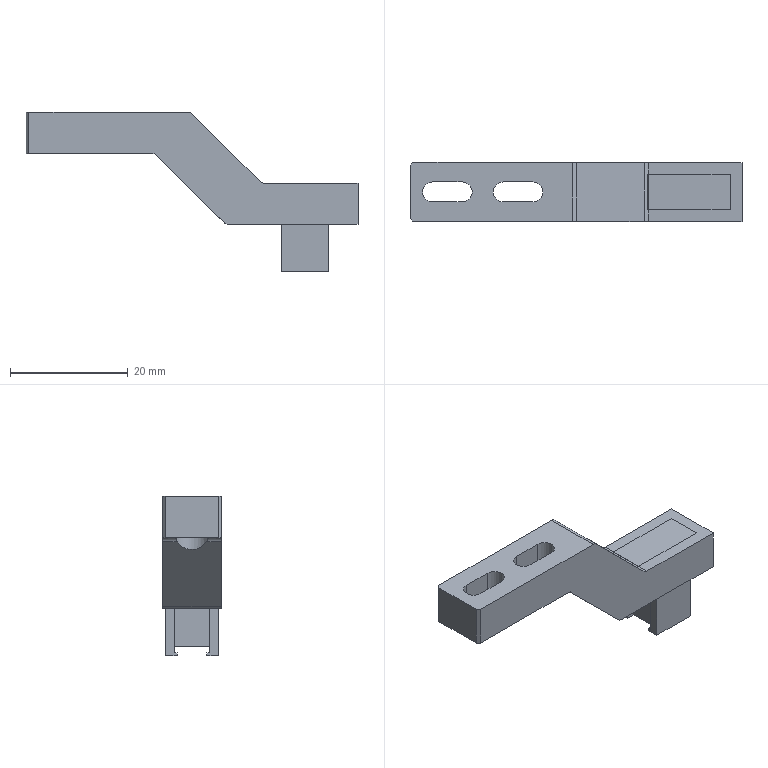NC program | NX | posted with a generic post | part box 56.3 x 10 x 27 mm
Lines 1606 to 2774 of 5717:
(ZLEVEL_PROFILE_COPY_1 , TOOL : D4R0.2)
N3174 T05 M6
N3176 G54
N3178 G17 G0 G90 X1.943 Y6.282 S9500 M3
N3180 G43 Z30. H5
N3182 Z1.487
N3184 G94 G1 Z-0.013 F800.
N3186 X1.426 Y5.877
N3188 G3 X1.277 Y5.505 R0.4
N3190 G1 X1.348 Y5. F2000.
N3192 Y-5.
N3194 X1.273 Y-5.514
N3196 X1.31 Y-5.517 Z-0.02
N3198 X1.346 Y-5.519 Z-0.028
N3200 X1.426 Y-5.
N3202 Y5.
N3204 X1.35 Y5.504
N3206 X1.4 Y5.502 Z-0.038
N3208 X1.439 Y5.5 Z-0.048
N3210 X1.507 Y5.055
N3212 Y5.
N3214 Y-5.
N3216 X1.444 Y-5.476
N3218 X1.433 Y-5.522
N3220 X1.474 Y-5.521 Z-0.062
N3222 X1.514 Y-5.52 Z-0.077
N3224 X1.592 Y-5.
N3226 Y5.
N3228 X1.589 Y5.055
N3230 X1.52 Y5.503
N3232 X1.563 Z-0.094
N3234 X1.605 Y5.504 Z-0.112
N3236 X1.67 Y5.055
N3238 X1.676 Y5.
N3240 Y-5.
N3242 X1.61 Y-5.476
N3244 X1.6 Y-5.515
N3246 X1.689 Y-5.505 Z-0.154
N3248 X1.758 Y-5.
N3250 Y5.
N3252 X1.69 Y5.501
N3254 X1.73 Z-0.179
N3256 X1.77 Z-0.203
N3258 X1.838 Y5.
N3260 Y-5.
N3262 X1.77 Y-5.501
N3264 X1.809 Z-0.231
N3266 X1.851 Z-0.26
N3268 X1.915 Y-5.
N3270 Y5.
N3272 X1.851 Y5.502
N3274 X1.886 Z-0.291
N3276 X1.926 Y5.501 Z-0.322
N3278 X1.988 Y5.
N3280 Y-5.
N3282 X1.93 Y-5.5
N3284 X1.977 Z-0.356
N3286 X2.013 Z-0.39
N3288 X2.058 Y-5.
N3290 Y5.
N3292 G3 X2.006 Y5.5 R16.197
N3294 G1 X2.043 Z-0.425
N3296 X2.08 Z-0.46
N3298 G2 X2.128 Y5. R21.014
N3300 G1 Y-5.
N3302 X2.086 Y-5.5
N3304 X2.124 Z-0.496
N3306 X2.159 Z-0.531
N3308 X2.199 Y-5.
N3310 Y5.
N3312 G3 X2.153 Y5.5 R26.18
N3314 G1 X2.19 Z-0.566
N3316 X2.227 Z-0.601
N3318 G2 X2.27 Y5. R24.032
N3320 G1 Y-5.
N3322 X2.232 Y-5.5
N3324 X2.27 Z-0.636
N3326 X2.305 Z-0.672
N3328 X2.341 Y-5.
N3330 Y5.
N3332 G3 X2.301 Y5.5 R39.219
N3334 G1 X2.338 Z-0.707
N3336 X2.374 Z-0.742
N3338 X2.412 Y5.
N3340 Y-5.
N3342 X2.378 Y-5.5
N3344 X2.416 Z-0.777
N3346 X2.451 Z-0.813
N3348 X2.482 Y-5.
N3350 Y5.
N3352 X2.448 Y5.5
N3354 X2.485 Z-0.848
N3356 X2.522 Z-0.883
N3358 X2.553 Y5.
N3360 Y-5.
N3362 X2.525 Y-5.5
N3364 X2.563 Z-0.918
N3366 X2.598 Z-0.954
N3368 X2.624 Y-5.
N3370 Y5.
N3372 X2.595 Y5.5
N3374 X2.633 Z-0.989
N3376 X2.669 Z-1.024
N3378 X2.695 Y5.
N3380 Y-5.
N3382 X2.671 Y-5.5
N3384 X2.709 Z-1.059
N3386 X2.744 Z-1.095
N3388 X2.766 Y-5.
N3390 Y5.
N3392 X2.742 Y5.5
N3394 X2.78 Z-1.13
N3396 X2.816 Z-1.165
N3398 X2.837 Y5.
N3400 Y-5.
N3402 X2.817 Y-5.5
N3404 X2.856 Z-1.2
N3406 X2.891 Z-1.236
N3408 X2.908 Y-5.
N3410 Y5.
N3412 X2.889 Y5.5
N3414 X2.926 Z-1.271
N3416 X2.962 Z-1.306
N3418 X2.979 Y5.
N3420 Y-5.
N3422 X2.964 Y-5.5
N3424 X3.002 Z-1.341
N3426 X3.037 Z-1.377
N3428 X3.05 Y-5.
N3430 Y5.
N3432 X3.035 Y5.5
N3434 X3.073 Z-1.412
N3436 X3.108 Z-1.447
N3438 X3.11 Y5.476
N3440 X3.121 Y5.
N3442 Y-5.
N3444 X3.11 Y-5.5
N3446 X3.148 Z-1.483
N3448 X3.183 Z-1.518
N3450 X3.192 Y-5.
N3452 Y5.
N3454 X3.18 Y5.5
N3456 X3.219 Z-1.553
N3458 X3.253 Z-1.588
N3460 X3.262 Y5.
N3462 Y-5.
N3464 X3.255 Y-5.5
N3466 X3.294 Z-1.624
N3468 X3.327 Z-1.659
N3470 X3.333 Y-5.
N3472 Y5.
N3474 X3.326 Y5.476
N3476 X3.325 Y5.5
N3478 X3.363 Z-1.694
N3480 X3.397 Z-1.729
N3482 X3.404 Y5.
N3484 Y-5.
N3486 X3.4 Y-5.5
N3488 X3.437 Z-1.765
N3490 X3.471 Z-1.8
N3492 X3.475 Y-5.
N3494 Y5.
N3496 X3.469 Y5.5
N3498 X3.505 Z-1.835
N3500 X3.54 Z-1.87
N3502 X3.546 Y5.
N3504 Y-5.
N3506 X3.542 Y-5.5
N3508 X3.579 Z-1.906
N3510 X3.613 Z-1.941
N3512 X3.617 Y-5.
N3514 Y5.
N3516 X3.611 Y5.5
N3518 X3.648 Z-1.976
N3520 X3.682 Z-2.011
N3522 X3.688 Y5.
N3524 Y-5.
N3526 X3.684 Y-5.5
N3528 X3.721 Z-2.047
N3530 X3.755 Z-2.082
N3532 X3.759 Y-5.
N3534 Y5.
N3536 X3.754 Y5.5
N3538 X3.79 Z-2.117
N3540 X3.825 Z-2.152
N3542 X3.83 Y5.
N3544 Y-5.
N3546 X3.826 Y-5.5
N3548 X3.863 Z-2.188
N3550 X3.897 Z-2.223
N3552 X3.901 Y-5.
N3554 Y5.
N3556 X3.896 Y5.5
N3558 X3.933 Z-2.258
N3560 X3.967 Z-2.293
N3562 X3.969 Y5.476
N3564 X3.972 Y5.
N3566 Y-5.
N3568 X3.97 Y-5.476
N3570 X3.968 Y-5.5
N3572 X4.005 Z-2.329
N3574 X4.04 Z-2.364
N3576 X4.041 Y-5.476
N3578 X4.042 Y-5.
N3580 Y5.
N3582 X4.04 Y5.476
N3584 X4.039 Y5.5
N3586 X4.075 Z-2.399
N3588 X4.11 Z-2.434
N3590 X4.111 Y5.476
N3592 X4.113 Y5.
N3594 Y-5.
N3596 X4.112 Y-5.476
N3598 X4.111 Y-5.5
N3600 X4.148 Z-2.47
N3602 X4.182 Z-2.505
N3604 X4.183 Y-5.476
N3606 X4.184 Y-5.
N3608 Y5.
N3610 X4.183 Y5.476
N3612 X4.181 Y5.5
N3614 X4.218 Z-2.54
N3616 X4.252 Z-2.575
N3618 X4.254 Y5.476
N3620 X4.255 Y5.
N3622 Y-5.
N3624 X4.254 Y-5.476
N3626 X4.253 Y-5.5
N3628 X4.29 Z-2.611
N3630 X4.324 Z-2.646
N3632 X4.325 Y-5.476
N3634 X4.326 Y-5.
N3636 Y5.
N3638 X4.325 Y5.476
N3640 X4.323 Y5.5
N3642 X4.36 Z-2.681
N3644 X4.395 Z-2.716
N3646 X4.396 Y5.476
N3648 X4.397 Y5.
N3650 Y-5.
N3652 X4.396 Y-5.476
N3654 X4.395 Y-5.5
N3656 X4.432 Z-2.752
N3658 X4.466 Z-2.787
N3660 X4.467 Y-5.476
N3662 X4.468 Y-5.
N3664 Y5.
N3666 X4.467 Y5.476
N3668 X4.466 Y5.5
N3670 X4.503 Z-2.822
N3672 X4.537 Z-2.857
N3674 X4.538 Y5.476
N3676 X4.539 Y5.
N3678 Y-5.
N3680 Y-5.476
N3682 X4.537 Y-5.5
N3684 X4.574 Z-2.893
N3686 X4.608 Z-2.928
N3688 X4.61 Y-5.476
N3690 Y-5.
N3692 Y5.
N3694 X4.609 Y5.476
N3696 X4.608 Y5.5
N3698 X4.645 Z-2.963
N3700 X4.679 Z-2.998
N3702 X4.68 Y5.476
N3704 X4.681 Y5.
N3706 Y-5.
N3708 X4.68 Y-5.476
N3710 X4.679 Y-5.5
N3712 X4.716 Z-3.034
N3714 X4.75 Z-3.069
N3716 X4.751 Y-5.476
N3718 X4.752 Y-5.
N3720 Y5.
N3722 X4.751 Y5.476
N3724 X4.75 Y5.5
N3726 X4.787 Z-3.104
N3728 X4.821 Z-3.14
N3730 X4.822 Y5.476
N3732 Y5.
N3734 Y-5.
N3736 Y-5.476
N3738 X4.821 Y-5.5
N3740 X4.858 Z-3.175
N3742 X4.892 Z-3.21
N3744 X4.893 Y-5.476
N3746 Y-5.
N3748 Y5.
N3750 Y5.476
N3752 X4.892 Y5.5
N3754 X4.929 Z-3.245
N3756 X4.963 Z-3.281
N3758 X4.964 Y5.476
N3760 Y5.
N3762 Y-5.
N3764 Y-5.476
N3766 X4.963 Y-5.5
N3768 X5. Z-3.316
N3770 X5.034 Z-3.351
N3772 X5.035 Y-5.476
N3774 Y-5.
N3776 Y5.
N3778 Y5.476
N3780 X5.033 Y5.5
N3782 X5.07 Z-3.386
N3784 X5.104 Z-3.422
N3786 X5.106 Y5.476
N3788 Y5.
N3790 Y-5.
N3792 Y-5.476
N3794 X5.105 Y-5.5
N3796 X5.141 Z-3.457
N3798 X5.175 Z-3.492
N3800 X5.177 Y-5.476
N3802 Y-5.
N3804 Y5.
N3806 Y5.476
N3808 X5.175 Y5.5
N3810 X5.212 Z-3.527
N3812 X5.246 Z-3.563
N3814 X5.248 Y5.476
N3816 Y5.
N3818 Y-5.
N3820 Y-5.476
N3822 X5.246 Y-5.5
N3824 X5.283 Z-3.598
N3826 X5.317 Z-3.633
N3828 X5.319 Y-5.476
N3830 Y-5.
N3832 Y5.
N3834 Y5.476
N3836 X5.317 Y5.5
N3838 X5.354 Z-3.668
N3840 X5.388 Z-3.704
N3842 X5.39 Y5.476
N3844 Y5.
N3846 Y-5.
N3848 Y-5.476
N3850 X5.388 Y-5.5
N3852 X5.425 Z-3.739
N3854 X5.459 Z-3.774
N3856 X5.461 Y-5.476
N3858 Y-5.
N3860 Y5.
N3862 Y5.476
N3864 X5.459 Y5.5
N3866 X5.496 Z-3.809
N3868 X5.53 Z-3.845
N3870 X5.531 Y5.476
N3872 X5.532 Y5.
N3874 Y-5.
N3876 Y-5.476
N3878 X5.53 Y-5.5
N3880 X5.567 Z-3.88
N3882 X5.601 Z-3.915
N3884 X5.602 Y-5.476
N3886 Y-5.
N3888 Y5.
N3890 Y5.476
N3892 X5.601 Y5.5
N3894 X5.638 Z-3.95
N3896 X5.672 Z-3.986
N3898 X5.673 Y5.476
N3900 Y5.
N3902 Y-5.
N3904 Y-5.476
N3906 X5.672 Y-5.5
N3908 X5.709 Z-4.021
N3910 X5.743 Z-4.056
N3912 X5.744 Y-5.476
N3914 Y-5.
N3916 Y5.
N3918 Y5.476
N3920 X5.743 Y5.5
N3922 X5.78 Z-4.091
N3924 X5.814 Z-4.127
N3926 X5.815 Y5.476
N3928 Y5.
N3930 Y-5.
N3932 Y-5.476
N3934 X5.814 Y-5.5
N3936 X5.851 Z-4.162
N3938 X5.885 Z-4.197
N3940 X5.886 Y-5.476
N3942 Y-5.
N3944 Y5.
N3946 Y5.476
N3948 X5.885 Y5.5
N3950 X5.922 Z-4.232
N3952 X5.956 Z-4.268
N3954 X5.957 Y5.476
N3956 Y5.
N3958 Y-5.
N3960 Y-5.476
N3962 X5.956 Y-5.5
N3964 X5.992 Z-4.303
N3966 X6.026 Z-4.338
N3968 X6.028 Y-5.476
N3970 Y-5.
N3972 Y5.
N3974 Y5.476
N3976 X6.026 Y5.5
N3978 X6.063 Z-4.373
N3980 X6.097 Z-4.409
N3982 X6.099 Y5.476
N3984 Y5.
N3986 Y-5.
N3988 Y-5.476
N3990 X6.097 Y-5.5
N3992 X6.134 Z-4.444
N3994 X6.168 Z-4.479
N3996 X6.17 Y-5.476
N3998 Y-5.
N4000 Y5.
N4002 Y5.476
N4004 X6.168 Y5.5
N4006 X6.205 Z-4.514
N4008 X6.24 Z-4.55
N4010 X6.241 Y5.
N4012 Y-5.
N4014 X6.24 Y-5.5
N4016 X6.276 Z-4.585
N4018 X6.31 Z-4.62
N4020 X6.312 Y-5.476
N4022 Y-5.
N4024 Y5.
N4026 Y5.476
N4028 X6.31 Y5.5
N4030 X6.347 Z-4.656
N4032 X6.381 Z-4.691
N4034 X6.382 Y5.476
N4036 Y5.
N4038 Y-5.
N4040 Y-5.476
N4042 X6.381 Y-5.5
N4044 X6.418 Z-4.726
N4046 X6.452 Z-4.761
N4048 X6.453 Y-5.476
N4050 Y-5.
N4052 Y5.
N4054 Y5.476
N4056 X6.452 Y5.5
N4058 X6.489 Z-4.797
N4060 X6.524 Z-4.832
N4062 Y5.
N4064 Y-5.
N4066 Y-5.5
N4068 X6.56 Z-4.867
N4070 X6.594 Z-4.902
N4072 X6.595 Y-5.476
N4074 Y-5.
N4076 Y5.
N4078 Y5.476
N4080 X6.594 Y5.5
N4082 X6.631 Z-4.938
N4084 X6.665 Z-4.973
N4086 X6.666 Y5.476
N4088 Y5.
N4090 Y-5.
N4092 Y-5.476
N4094 X6.665 Y-5.5
N4096 X6.702 Z-5.008
N4098 X6.736 Z-5.043
N4100 X6.737 Y-5.476
N4102 Y-5.
N4104 Y5.
N4106 Y5.476
N4108 X6.736 Y5.5
N4110 X6.772 Z-5.079
N4112 X6.807 Z-5.114
N4114 X6.808 Y5.
N4116 Y-5.
N4118 X6.807 Y-5.5
N4120 X6.843 Z-5.149
N4122 X6.877 Z-5.184
N4124 X6.879 Y-5.476
N4126 Y-5.
N4128 Y5.
N4130 Y5.476
N4132 X6.877 Y5.5
N4134 X6.914 Z-5.22
N4136 X6.948 Z-5.255
N4138 X6.95 Y5.476
N4140 Y5.
N4142 Y-5.
N4144 Y-5.476
N4146 X6.948 Y-5.5
N4148 X6.985 Z-5.29
N4150 X7.019 Z-5.325
N4152 X7.021 Y-5.476
N4154 Y-5.
N4156 Y5.
N4158 Y5.476
N4160 X7.019 Y5.5
N4162 X7.056 Z-5.361
N4164 X7.09 Z-5.396
N4166 X7.092 Y5.
N4168 Y-5.
N4170 X7.09 Y-5.5
N4172 X7.127 Z-5.431
N4174 X7.161 Z-5.466
N4176 X7.162 Y-5.476
N4178 Y-5.
N4180 Y5.
N4182 Y5.476
N4184 X7.161 Y5.5
N4186 X7.198 Z-5.502
N4188 X7.232 Z-5.537
N4190 X7.233 Y5.476
N4192 Y5.
N4194 Y-5.
N4196 Y-5.476
N4198 X7.232 Y-5.5
N4200 X7.269 Z-5.572
N4202 X7.303 Z-5.607
N4204 X7.304 Y-5.476
N4206 Y-5.
N4208 Y5.
N4210 Y5.476
N4212 X7.303 Y5.5
N4214 X7.34 Z-5.643
N4216 X7.374 Z-5.678
N4218 X7.375 Y5.
N4220 Y-5.
N4222 X7.374 Y-5.5
N4224 X7.411 Z-5.713
N4226 X7.445 Z-5.748
N4228 X7.446 Y-5.476
N4230 Y5.
N4232 Y5.476
N4234 X7.445 Y5.5
N4236 X7.482 Z-5.784
N4238 X7.516 Z-5.819
N4240 X7.517 Y5.476
N4242 Y5.
N4244 Y-5.
N4246 Y-5.476
N4248 X7.516 Y-5.5
N4250 X7.552 Z-5.854
N4252 X7.587 Z-5.889
N4254 X7.588 Y-5.476
N4256 Y-5.
N4258 Y5.
N4260 Y5.476
N4262 X7.587 Y5.5
N4264 X7.623 Z-5.925
N4266 X7.658 Z-5.96
N4268 X7.659 Y5.
N4270 Y-5.
N4272 X7.658 Y-5.5
N4274 X7.694 Z-5.995
N4276 X7.728 Z-6.03
N4278 X7.73 Y-5.476
N4280 Y-5.
N4282 Y5.
N4284 Y5.476
N4286 X7.728 Y5.5
N4288 X7.765 Z-6.066
N4290 X7.799 Z-6.101
N4292 X7.801 Y5.476
N4294 Y5.
N4296 Y-5.
N4298 Y-5.476
N4300 X7.799 Y-5.5
N4302 X7.836 Z-6.136
N4304 X7.87 Z-6.171
N4306 X7.872 Y-5.476
N4308 Y-5.
N4310 Y5.
N4312 Y5.476
N4314 X7.87 Y5.5
N4316 X7.907 Z-6.207
N4318 X7.941 Z-6.242
N4320 X7.942 Y5.
N4322 Y-5.
N4324 X7.941 Y-5.5
N4326 X7.978 Z-6.277
N4328 X8.012 Z-6.313
N4330 X8.013 Y-5.476
N4332 Y-5.
N4334 Y5.
N4336 Y5.476
N4338 X8.012 Y5.5
N4340 X8.049 Z-6.348
N4342 X8.083 Z-6.383
N4344 X8.084 Y5.476
N4346 Y-5.
N4348 Y-5.476
N4350 X8.083 Y-5.5
N4352 X8.12 Z-6.418
N4354 X8.154 Z-6.454
N4356 X8.155 Y-5.476
N4358 Y-5.
N4360 Y5.
N4362 Y5.476
N4364 X8.154 Y5.5
N4366 X8.191 Z-6.489
N4368 X8.225 Z-6.524
N4370 X8.226 Y5.
N4372 Y-5.
N4374 X8.225 Y-5.5
N4376 X8.262 Z-6.559
N4378 X8.296 Z-6.595
N4380 X8.297 Y-5.476
N4382 Y-5.
N4384 Y5.
N4386 Y5.476
N4388 X8.296 Y5.5
N4390 X8.332 Z-6.63
N4392 X8.367 Z-6.665
N4394 X8.368 Y5.476
N4396 Y5.
N4398 Y-5.
N4400 Y-5.476
N4402 X8.367 Y-5.5
N4404 X8.403 Z-6.7
N4406 X8.437 Z-6.736
N4408 X8.439 Y-5.476
N4410 Y-5.
N4412 Y5.
N4414 Y5.476
N4416 X8.437 Y5.5
N4418 X8.474 Z-6.771
N4420 X8.508 Z-6.806
N4422 X8.51 Y5.476
N4424 Y5.
N4426 Y-5.
N4428 Y-5.476
N4430 X8.508 Y-5.5
N4432 X8.545 Z-6.841
N4434 X8.579 Z-6.877
N4436 X8.581 Y-5.476
N4438 Y-5.
N4440 Y5.
N4442 Y5.476
N4444 X8.579 Y5.5
N4446 X8.616 Z-6.912
N4448 X8.65 Z-6.947
N4450 X8.652 Y5.476
N4452 Y5.
N4454 Y-5.
N4456 Y-5.476
N4458 X8.65 Y-5.5
N4460 X8.687 Z-6.982
N4462 X8.721 Z-7.018
N4464 X8.722 Y-5.476
N4466 Y-5.
N4468 Y5.
N4470 Y5.476
N4472 X8.721 Y5.5
N4474 X8.758 Z-7.053
N4476 X8.792 Z-7.088
N4478 X8.793 Y5.476
N4480 Y5.
N4482 Y-5.
N4484 Y-5.476
N4486 X8.792 Y-5.5
N4488 X8.829 Z-7.123
N4490 X8.863 Z-7.159
N4492 X8.864 Y-5.476
N4494 Y-5.
N4496 Y5.
N4498 Y5.476
N4500 X8.863 Y5.5
N4502 X8.9 Z-7.194
N4504 X8.934 Z-7.229
N4506 X8.935 Y5.476
N4508 Y5.
N4510 Y-5.
N4512 Y-5.476
N4514 X8.934 Y-5.5
N4516 X8.971 Z-7.264
N4518 X9.005 Z-7.3
N4520 X9.006 Y-5.476
N4522 Y-5.
N4524 Y5.
N4526 Y5.476
N4528 X9.005 Y5.5
N4530 X9.042 Z-7.335
N4532 X9.076 Z-7.37
N4534 X9.077 Y5.476
N4536 Y5.
N4538 Y-5.
N4540 Y-5.476
N4542 X9.076 Y-5.5
N4544 X9.113 Z-7.405
N4546 X9.147 Z-7.441
N4548 X9.148 Y-5.476
N4550 Y-5.
N4552 Y5.
N4554 Y5.476
N4556 X9.147 Y5.5
N4558 X9.183 Z-7.476
N4560 X9.217 Z-7.511
N4562 X9.219 Y5.476
N4564 Y5.
N4566 Y-5.
N4568 Y-5.476
N4570 X9.217 Y-5.5
N4572 X9.254 Z-7.546
N4574 X9.288 Z-7.582
N4576 X9.29 Y-5.476
N4578 Y-5.
N4580 Y5.
N4582 Y5.476
N4584 X9.288 Y5.5
N4586 X9.325 Z-7.617
N4588 X9.359 Z-7.652
N4590 X9.361 Y5.476
N4592 Y5.
N4594 Y-5.
N4596 Y-5.476
N4598 X9.359 Y-5.5
N4600 X9.396 Z-7.687
N4602 X9.43 Z-7.723
N4604 X9.432 Y-5.476
N4606 Y-5.
N4608 Y5.
N4610 Y5.476
N4612 X9.43 Y5.5
N4614 X9.467 Z-7.758
N4616 X9.501 Z-7.793
N4618 X9.503 Y5.476
N4620 X9.502 Y5.
N4622 Y-5.
N4624 X9.503 Y-5.476
N4626 X9.501 Y-5.5
N4628 X9.538 Z-7.829
N4630 X9.572 Z-7.864
N4632 X9.573 Y-5.476
N4634 Y-5.
N4636 Y5.
N4638 Y5.476
N4640 X9.572 Y5.5
N4642 X9.609 Z-7.899
N4644 X9.643 Z-7.934
N4646 X9.644 Y5.476
N4648 Y5.
N4650 Y-5.
N4652 Y-5.476
N4654 X9.643 Y-5.5
N4656 X9.68 Z-7.97
N4658 X9.714 Z-8.005
N4660 X9.715 Y-5.476
N4662 Y-5.
N4664 Y5.
N4666 Y5.476
N4668 X9.714 Y5.5
N4670 X9.751 Z-8.04
N4672 X9.785 Z-8.075
N4674 X9.786 Y5.476
N4676 Y5.
N4678 Y-5.
N4680 Y-5.476
N4682 X9.785 Y-5.5
N4684 X9.822 Z-8.111
N4686 X9.856 Z-8.146
N4688 X9.857 Y-5.476
N4690 Y-5.
N4692 Y5.
N4694 Y5.476
N4696 X9.856 Y5.5
N4698 X9.893 Z-8.181
N4700 X9.927 Z-8.216
N4702 X9.928 Y5.476
N4704 Y5.
N4706 Y-5.
N4708 Y-5.476
N4710 X9.927 Y-5.5
N4712 X9.964 Z-8.252
N4714 X9.998 Z-8.287
N4716 X9.999 Y-5.476
N4718 Y-5.
N4720 Y5.
N4722 Y5.476
N4724 X9.997 Y5.5
N4726 X10.034 Z-8.322
N4728 X10.068 Z-8.357
N4730 X10.07 Y5.476
N4732 Y5.
N4734 Y-5.
N4736 Y-5.476
N4738 X10.068 Y-5.5
N4740 X10.105 Z-8.393
N4742 X10.139 Z-8.428
N4744 X10.141 Y-5.476
N4746 Y-5.
N4748 Y5.
N4750 Y5.476
N4752 X10.139 Y5.5
N4754 X10.176 Z-8.463
N4756 X10.21 Z-8.498
N4758 X10.212 Y5.476
N4760 Y5.
N4762 Y-5.
N4764 Y-5.476
N4766 X10.21 Y-5.5
N4768 X10.247 Z-8.534
N4770 X10.281 Z-8.569
N4772 X10.283 Y-5.476
N4774 Y-5.
N4776 Y5.
N4778 Y5.476
N4780 X10.281 Y5.5
N4782 X10.318 Z-8.604
N4784 X10.352 Z-8.639
N4786 X10.354 Y5.476
N4788 X10.353 Y5.
N4790 Y-5.
N4792 X10.354 Y-5.476
N4794 X10.352 Y-5.5
N4796 X10.389 Z-8.675
N4798 X10.423 Z-8.71
N4800 X10.425 Y-5.476
N4802 X10.424 Y-5.
N4804 Y5.
N4806 Y5.476
N4808 X10.423 Y5.5
N4810 X10.46 Z-8.745
N4812 X10.494 Z-8.78
N4814 X10.495 Y5.476
N4816 Y5.
N4818 Y-5.
N4820 Y-5.476
N4822 X10.494 Y-5.5
N4824 X10.531 Z-8.816
N4826 X10.565 Z-8.851
N4828 X10.566 Y-5.476
N4830 Y-5.
N4832 Y5.
N4834 Y5.476
N4836 X10.565 Y5.5
N4838 X10.602 Z-8.886
N4840 X10.636 Z-8.921
N4842 X10.637 Y5.476
N4844 Y5.
N4846 Y-5.
N4848 Y-5.476
N4850 X10.636 Y-5.5
N4852 X10.673 Z-8.957
N4854 X10.707 Z-8.992
N4856 X10.708 Y-5.476
N4858 Y-5.
N4860 Y5.
N4862 Y5.476
N4864 X10.707 Y5.5
N4866 X10.744 Z-9.027
N4868 X10.778 Z-9.062
N4870 X10.779 Y5.476
N4872 Y5.
N4874 Y-5.
N4876 Y-5.476
N4878 X10.778 Y-5.5
N4880 X10.815 Z-9.098
N4882 X10.849 Z-9.133
N4884 X10.85 Y-5.476
N4886 Y-5.
N4888 Y5.
N4890 Y5.476
N4892 X10.849 Y5.5
N4894 X10.885 Z-9.168
N4896 X10.92 Z-9.203
N4898 X10.921 Y5.476
N4900 Y5.
N4902 Y-5.
N4904 Y-5.476
N4906 X10.92 Y-5.5
N4908 X10.957 Z-9.239
N4910 X10.991 Z-9.274
N4912 X10.992 Y-5.476
N4914 Y-5.
N4916 Y5.
N4918 Y5.476
N4920 X10.991 Y5.5
N4922 X11.027 Z-9.309
N4924 X11.062 Z-9.344
N4926 X11.063 Y5.476
N4928 Y5.
N4930 Y-5.
N4932 Y-5.476
N4934 X11.062 Y-5.5
N4936 X11.099 Z-9.38
N4938 X11.133 Z-9.415
N4940 X11.135 Y-5.476
N4942 X11.133 Y-5.
N4944 Y5.
N4946 X11.134 Y5.476
N4948 X11.133 Y5.5
N4950 X11.17 Z-9.45
N4952 X11.204 Z-9.486
N4954 X11.205 Y5.476
N4956 X11.204 Y5.
N4958 Y-5.
N4960 X11.206 Y-5.476
N4962 X11.204 Y-5.5
N4964 X11.242 Z-9.521
N4966 X11.276 Z-9.556
N4968 X11.277 Y-5.476
N4970 X11.275 Y-5.
N4972 Y5.
N4974 X11.276 Y5.476
N4976 X11.275 Y5.5
N4978 X11.312 Z-9.591
N4980 X11.346 Z-9.627
N4982 X11.347 Y5.476
N4984 X11.346 Y5.
N4986 Y-5.
N4988 X11.348 Y-5.476
N4990 X11.347 Y-5.5
N4992 X11.384 Z-9.662
N4994 X11.418 Z-9.697
N4996 X11.42 Y-5.476
N4998 X11.417 Y-5.
N5000 Y5.
N5002 X11.418 Y5.476
N5004 X11.417 Y5.5
N5006 X11.454 Z-9.732
N5008 X11.488 Z-9.768
N5010 X11.489 Y5.476
N5012 X11.488 Y5.
N5014 Y-5.
N5016 X11.491 Y-5.476
N5018 X11.489 Y-5.5
N5020 X11.527 Z-9.803
N5022 X11.561 Z-9.838
N5024 X11.562 Y-5.476
N5026 X11.559 Y-5.
N5028 Y5.
N5030 Y5.5
N5032 X11.596 Z-9.873
N5034 X11.63 Z-9.909
N5036 Y5.
N5038 Y-5.
N5040 X11.633 Y-5.476
N5042 X11.632 Y-5.5
N5044 X11.669 Z-9.944
N5046 X11.703 Z-9.979
N5048 X11.705 Y-5.476
N5050 X11.701 Y-5.
N5052 Y5.
N5054 Y5.5
N5056 X11.738 Z-10.014
N5058 X11.772 Z-10.05
N5060 Y5.
N5062 Y-5.
N5064 X11.776 Y-5.476
N5066 X11.774 Y-5.5
N5068 X11.812 Z-10.085
N5070 X11.846 Z-10.12
N5072 X11.847 Y-5.476
N5074 X11.843 Y-5.
N5076 Y5.
N5078 Y5.5
N5080 X11.88 Z-10.155
N5082 X11.915 Z-10.191
N5084 X11.913 Y5.
N5086 Y-5.
N5088 X11.918 Y-5.476
N5090 X11.917 Y-5.5
N5092 X11.954 Z-10.226
N5094 X11.988 Z-10.261
N5096 X11.99 Y-5.476
N5098 X11.984 Y-5.
N5100 Y5.
N5102 X11.987 Y5.476
N5104 X11.986 Y5.5
N5106 X12.023 Z-10.296
N5108 X12.057 Z-10.332
N5110 X12.058 Y5.476
N5112 X12.055 Y5.
N5114 Y-5.
N5116 X12.061 Y-5.476
N5118 X12.059 Y-5.5
N5120 X12.097 Z-10.367
N5122 X12.131 Z-10.402
N5124 X12.132 Y-5.476
N5126 X12.126 Y-5.
N5128 Y5.
N5130 X12.129 Y5.476
N5132 X12.128 Y5.5
N5134 X12.165 Z-10.437
N5136 X12.2 Z-10.473
N5138 X12.201 Y5.476
N5140 X12.197 Y5.
N5142 Y-5.
N5144 X12.204 Y-5.476
N5146 X12.203 Y-5.5
N5148 X12.24 Z-10.508
N5150 X12.276 Z-10.543
N5152 X12.277 Y-5.476
N5154 X12.268 Y-5.
N5156 Y5.
N5158 X12.272 Y5.5
N5160 X12.309 Z-10.578
N5162 X12.345 Z-10.614
N5164 X12.347 Y5.476
N5166 X12.339 Y5.
N5168 Y-5.
N5170 X12.349 Y-5.5
N5172 X12.387 Z-10.649
N5174 X12.423 Z-10.684
N5176 X12.424 Y-5.476
N5178 X12.41 Y-5.
N5180 Y5.
N5182 X12.418 Y5.5
N5184 X12.456 Z-10.719
N5186 X12.491 Z-10.755
N5188 X12.486 Y4.935
N5190 X12.481 Y4.926
N5192 Y-5.
N5194 X12.496 Y-5.5
N5196 X12.535 Z-10.79
N5198 X12.57 Z-10.825
N5200 X12.552 Y-5.
N5202 Y4.897
N5204 X12.557 Y4.915
N5206 X12.564 Y5.5
N5208 X12.602 Z-10.86
N5210 X12.637 Z-10.896
N5212 X12.639 Y5.476
N5214 X12.628 Y4.903
N5216 X12.623 Y4.887
N5218 Y-5.
N5220 X12.645 Y-5.476
N5222 X12.644 Y-5.5
N5224 X12.682 Z-10.931
N5226 X12.717 Z-10.966
N5228 X12.693 Y-5.
N5230 Y4.877
N5232 X12.702 Y4.915
N5234 X12.712 Y5.476
N5236 X12.711 Y5.5
N5238 X12.749 Z-11.002
N5240 X12.784 Z-11.037
N5242 X12.77 Y4.884
N5244 X12.764 Y4.87
N5246 Y-5.
N5248 X12.791 Y-5.5
N5250 X12.83 Z-11.072
N5252 X12.865 Z-11.107
N5254 X12.835 Y-5.
N5256 Y4.865
N5258 X12.841 Y4.879
N5260 X12.857 Y5.5
N5262 X12.895 Z-11.143
N5264 X12.93 Z-11.178
N5266 X12.912 Y4.874
N5268 X12.906 Y4.86
N5270 Y-5.
N5272 X12.939 Y-5.5
N5274 X12.977 Z-11.213
N5276 X13.012 Z-11.248
N5278 X13.014 Y-5.476
N5280 X12.983 Y-4.98
N5282 X12.977 Y-4.964
N5284 Y4.855
N5286 X12.983 Y4.869
N5288 X13.005 Y5.476
N5290 X13.004 Y5.5
N5292 X13.042 Z-11.284
N5294 X13.077 Z-11.319
N5296 X13.06 Y4.915
N5298 X13.048 Y4.852
N5300 Y-4.961
N5302 X13.054 Y-4.97
N5304 X13.088 Y-5.476
N5306 X13.086 Y-5.5
N5308 X13.125 Z-11.354
N5310 X13.16 Z-11.389
N5312 X13.161 Y-5.476
N5314 X13.125 Y-4.957
N5316 X13.119 Y-4.948
N5318 Y4.852
N5320 X13.132 Y4.915
N5322 X13.15 Y5.5
N5324 X13.188 Z-11.425
N5326 X13.223 Z-11.46
N5328 X13.225 Y5.476
N5330 X13.203 Y4.915
N5332 X13.19 Y4.852
N5334 Y-4.934
N5336 X13.234 Y-5.5
N5338 X13.272 Z-11.495
N5340 X13.308 Z-11.53
N5342 X13.261 Y-4.92
N5344 Y4.852
N5346 G3 X13.296 Y5.5 R2.892
N5348 G1 X13.334 Z-11.565
N5350 X13.374 Z-11.6
N5352 G2 X13.33 Y4.856 R2.482
N5354 G1 Y-4.9
N5356 X13.336 Y-4.915
N5358 X13.384 Y-5.5
N5360 X13.417 Z-11.633
N5362 X13.458 Z-11.667
N5364 G3 X13.398 Y-4.893 R2.572
N5366 G1 Y4.86
N5368 G3 X13.449 Y5.5 R2.17
N5370 G1 X13.474 Z-11.7
N5372 X13.523 Z-11.733
N5374 G2 X13.464 Y4.849 R1.962
N5376 G1 Y-4.885
N5378 G2 X13.531 Y-5.5 R2.116
N5380 G1 X13.563 Z-11.764
N5382 X13.605 Z-11.796
N5384 X13.558 Y-4.89
N5386 X13.529 Y-4.794
N5388 Y4.761
N5390 G3 X13.597 Y5.5 R2.645
N5392 G1 X13.633 Y5.499 Z-11.821
N5394 X13.679 Z-11.847
N5396 G2 X13.592 Y4.74 R2.126
N5398 G1 Y-4.754
N5400 G2 X13.679 Y-5.499 R2.085
N5402 G1 X13.707 Z-11.869
N5404 X13.751 Z-11.892
N5406 G3 X13.661 Y-4.707 R2.192
N5408 G1 Y4.71
N5410 X13.688 Y4.76
N5412 X13.76 Y5.499
N5414 X13.801 Z-11.909
N5416 X13.838 Y5.5 Z-11.926
N5418 X13.75 Y4.746
N5420 X13.726 Y4.696
N5422 Y-4.666
N5424 G2 X13.821 Y-5.499 R2.225
N5426 G1 X13.874 Z-11.95
N5428 G3 X13.785 Y-4.702 R2.083
N5430 G1 Y4.714
N5432 X13.802 Y4.748
N5434 X13.901 Y5.476
N5436 X13.9 Y5.492
N5438 X13.947 Y5.48 Z-11.966
N5440 X13.868 Y4.821
N5442 X13.834 Y4.749
N5444 Y-4.719
N5446 X13.868 Y-4.794
N5448 X13.934 Y-5.476
N5450 X13.933 Y-5.49
N5452 X13.947 Y-5.487 Z-11.973
N5454 X13.983 Y-5.482 Z-11.98
N5456 G3 X13.886 Y-4.73 R1.608
N5458 G1 Y4.764
N5460 X13.927 Y4.835
N5462 X13.991 Y5.341
N5464 X13.999 Z-11.984
N5466 X14.017 Y5.339 Z-11.987
N5468 G2 X13.921 Y4.804 R1.313
N5470 G1 Y-4.751
N5472 G2 X14.009 Y-5.478 R1.417
N5474 G1 X14.029 Y-5.36 Z-11.99
N5476 X14.044 Y-5.241 Z-11.994
N5478 X14.061 Y-5.122 Z-11.997
N5480 X14.06 Y-5.005 Z-12.
N5482 G3 X14. Y-4.743 R2.245
N5484 G1 Y-2.986
N5486 G3 X14.256 Y-2.791 R0.429
N5488 G2 X14.107 Y2.85 R20.443
N5490 G1 X14. Y3.
N5492 Y4.93
N5494 X14.034 Y4.99
N5496 G2 X14.377 Y5.195 R0.4
N5498 G1 X14.928 Y5.203
N5500 Z-10.5
N5502 G0 Z30.
N5504 M5